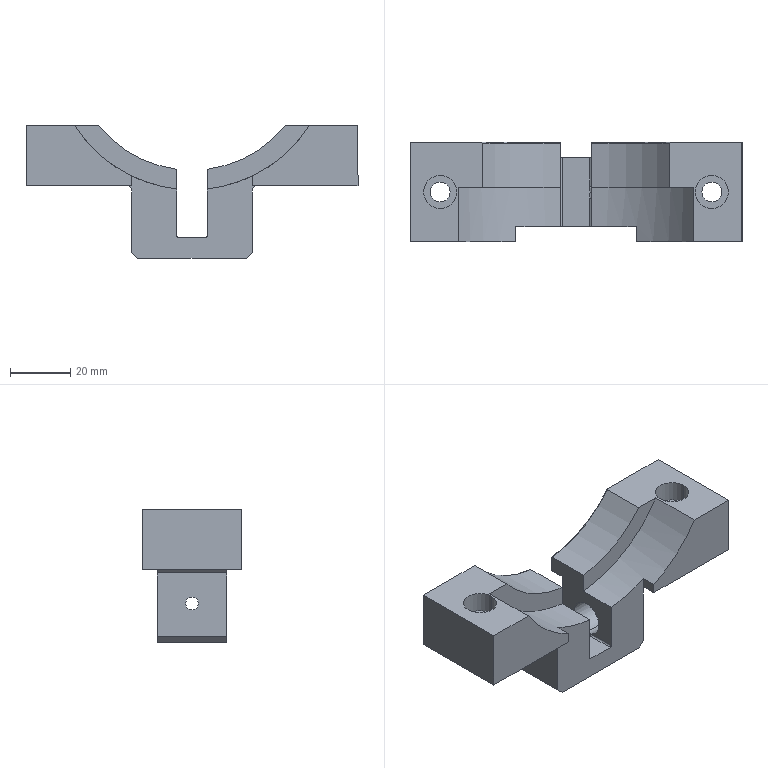Part | STEP file | PN_0019 Default | 1 solid | 59 faces | box 110 x 33 x 44 mm | volume 53876 mm3 | plane 31 | cylinder 25 | cone 2 | spline 1 | commonest cylinder face diameters 6.6 x4 11 x4 13 x4 1 x3 4.2 x2 5 x2